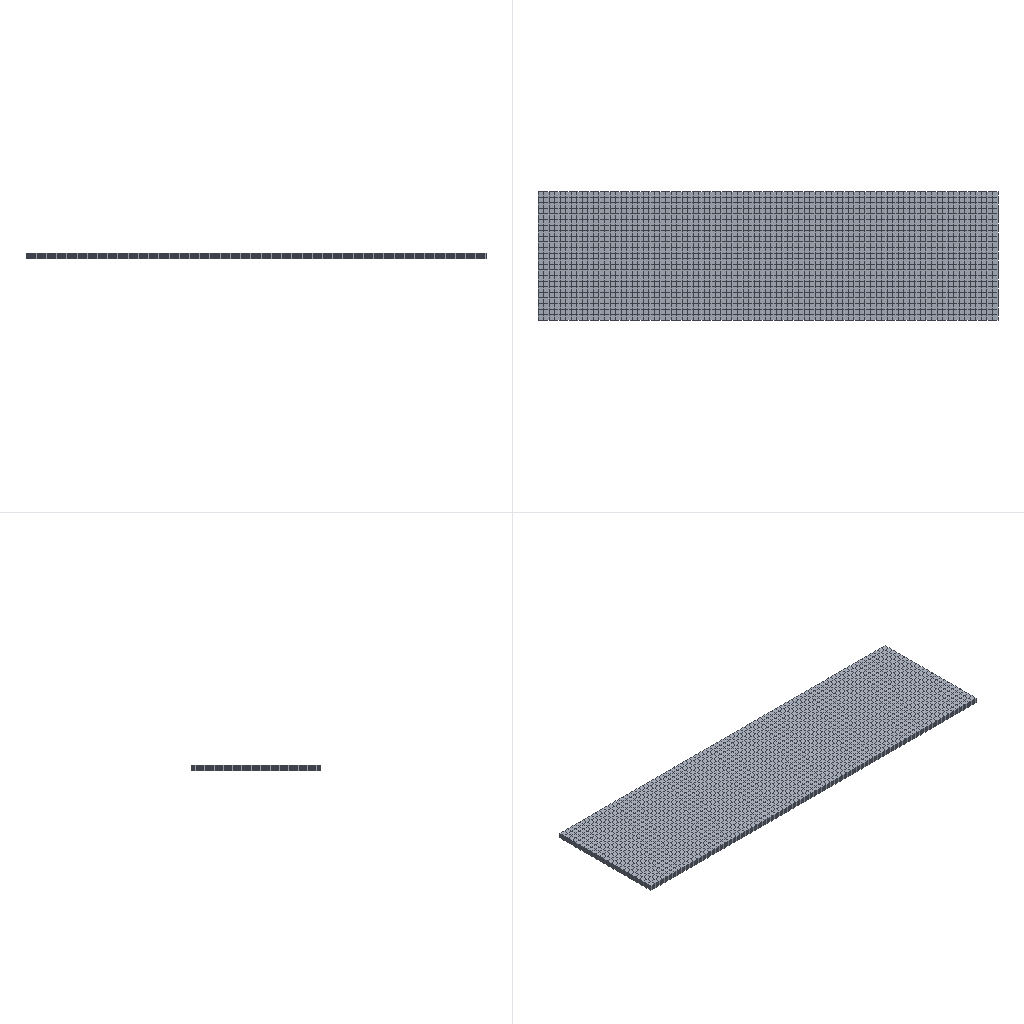Simulation study | abaqus
Set-up summary:
category,name,step,type,value,unit,region
solver,abaqus
solver,version,,,Abaqus/Standard 3DEXPERIENCE R2017x
units,not stated in the deck,,not stated
analysis,deck,,thermal,thermal
load_step,step,step,thermal
load_step,requested,,,1
mesh,nodes,,,12096
mesh,elements,,,9545
element_type,DC3D8,,solid,9545
load,load commands in deck,,count,3
bc,support commands in deck,,count,1
material,SS316,,in results
check,setup vs results,,match,"per instance, exact: element labels, types and connectivity; labels of the nodes the elements use; coordinates of those nodes at SINGLE_PRECISION in 1 of 1 instance(s)"
Abaqus input file, long lists of numbers shortened:
*Heading
** Job name: Job-1 Model name: Job-forming
** Generated by: Abaqus/CAE 2017
*Preprint, echo=NO, model=NO, history=NO, contact=NO
**
** PARTS
**
*Part, name=work
*Node
      1,        1250.,        -350.,          15.
      2,   1234.94,        -350.,          15.
** (12094 more lines like these left out)
*Element, type=DC3D8
   1,   505,   506,   590,   589,     1,     2,    86,    85
   2,   506,   507,   591,   590,     2,     3,    87,    86
** (9543 more lines like these left out)
*Nset, nset=Set-3, generate
     1,  12096,      1
*Elset, elset=Set-3, generate
    1,  9545,     1
** Section: Section-1
*Solid Section, elset=Set-3, material=ss316
,
*End Part
**
**
** ASSEMBLY
**
*Assembly, name=Assembly
**
*Instance, name=work-1, part=work
*End Instance
**
*Nset, nset=Set-32, instance=work-1, generate
     1,  12096,      1
*Elset, elset=Set-32, instance=work-1, generate
    1,  9545,     1
*Nset, nset=Set-48, instance=work-1, generate
     1,  12096,      1
*Elset, elset=Set-48, instance=work-1, generate
    1,  9545,     1
*Nset, nset=Set-49, instance=work-1
     1,     2,     3,     4,     5,     6,     7,     8,     9,    10,    11,    12,    13,    14,    15,    16
    17,    18,    19,    20,    21,    22,    23,    24,    25,    26,    27,    28,    29,    30,    31,    32
** (61 more lines like these left out)
*Elset, elset=Set-49, instance=work-1
    1,    2,    3,    4,    5,    6,    7,    8,    9,   10,   11,   12,   13,   14,   15,   16
   17,   18,   19,   20,   21,   22,   23,   24,   25,   26,   27,   28,   29,   30,   31,   32
** (50 more lines like these left out)
*Nset, nset=Set-50, instance=work-1, generate
     1,  12096,      1
*Elset, elset=Set-50, instance=work-1, generate
    1,  9545,     1
*Elset, elset=_Surf-37_S1, internal, instance=work-1, generate
 9131,  9545,     1
*Elset, elset=_Surf-37_S6, internal, instance=work-1, generate
    1,  9463,    83
*Elset, elset=_Surf-37_S2, internal, instance=work-1, generate
   1,  415,    1
*Elset, elset=_Surf-37_S4, internal, instance=work-1, generate
   83,  9545,    83
*Elset, elset=_Surf-37_S3, internal, instance=work-1
    1,    2,    3,    4,    5,    6,    7,    8,    9,   10,   11,   12,   13,   14,   15,   16
   17,   18,   19,   20,   21,   22,   23,   24,   25,   26,   27,   28,   29,   30,   31,   32
** (118 more lines like these left out)
*Elset, elset=_Surf-37_S5, internal, instance=work-1
  333,  334,  335,  336,  337,  338,  339,  340,  341,  342,  343,  344,  345,  346,  347,  348
  349,  350,  351,  352,  353,  354,  355,  356,  357,  358,  359,  360,  361,  362,  363,  364
** (118 more lines like these left out)
*Surface, type=ELEMENT, name=Surf-37
_Surf-37_S1, S1
_Surf-37_S6, S6
_Surf-37_S2, S2
_Surf-37_S4, S4
_Surf-37_S3, S3
_Surf-37_S5, S5
*Elset, elset=_Surf-38_S1, internal, instance=work-1, generate
 9131,  9545,     1
*Elset, elset=_Surf-38_S6, internal, instance=work-1, generate
    1,  9463,    83
*Elset, elset=_Surf-38_S2, internal, instance=work-1, generate
   1,  415,    1
*Elset, elset=_Surf-38_S4, internal, instance=work-1, generate
   83,  9545,    83
*Elset, elset=_Surf-38_S3, internal, instance=work-1
    1,    2,    3,    4,    5,    6,    7,    8,    9,   10,   11,   12,   13,   14,   15,   16
   17,   18,   19,   20,   21,   22,   23,   24,   25,   26,   27,   28,   29,   30,   31,   32
** (118 more lines like these left out)
*Elset, elset=_Surf-38_S5, internal, instance=work-1
  333,  334,  335,  336,  337,  338,  339,  340,  341,  342,  343,  344,  345,  346,  347,  348
  349,  350,  351,  352,  353,  354,  355,  356,  357,  358,  359,  360,  361,  362,  363,  364
** (118 more lines like these left out)
*Surface, type=ELEMENT, name=Surf-38
_Surf-38_S1, S1
_Surf-38_S6, S6
_Surf-38_S2, S2
_Surf-38_S4, S4
_Surf-38_S3, S3
_Surf-38_S5, S5
*End Assembly
*Amplitude, name=Amp-1
             0.,              1.,             0.1,              1.
**
** MATERIALS
**
*Material, name=ss316
*Conductivity
 13.31,  20.
 16.33, 200.
 19.47, 400.
 22.38, 600.
 25.07, 800.
 26.33, 900.
 27.53,1000.
 28.67,1100.
 29.76,1200.
 31.95,1420.
  320.,1460.
*Density
 7.966e-09,  20.
 7.893e-09, 200.
 7.814e-09, 400.
 7.724e-09, 600.
  7.63e-09, 800.
 7.583e-09, 900.
 7.535e-09,1000.
 7.486e-09,1100.
 7.436e-09,1200.
  7.32e-09,1420.
  7.32e-09,1460.
*Elastic
195100., 0.267,   20.
185700.,  0.29,  200.
172600.,   0.3,  400.
155000., 0.296,  600.
131400., 0.262,  800.
116800.,  0.24,  900.
100100., 0.229, 1000.
 81100., 0.223, 1100.
 59500., 0.223, 1200.
  2000., 0.223, 1420.
  2000., 0.223, 1460.
*Expansion
 1.524e-05,  20.
 1.643e-05, 200.
 1.744e-05, 400.
 1.821e-05, 600.
 1.883e-05, 800.
 1.911e-05, 900.
 1.938e-05,1000.
 1.966e-05,1100.
 1.995e-05,1200.
  2.07e-05,1420.
  2.07e-05,1460.
*Plastic
278.,   0.,  20.
325., 0.01,  20.
193.,   0., 200.
226., 0.01, 200.
154.,   0., 400.
180., 0.01, 400.
141.,   0., 600.
165., 0.01, 600.
130.,   0., 800.
153., 0.01, 800.
 86.,   0., 900.
100., 0.01, 900.
 45.,   0.,1000.
 53., 0.01,1000.
 22.,   0.,1100.
 23., 0.01,1100.
 13.,   0.,1200.
 15., 0.01,1200.
  3.,   0.,1420.
 3.3, 0.01,1420.
  3.,   0.,1460.
 3.3, 0.01,1460.
*Specific Heat
  4.7e+08,  20.
 5.08e+08, 200.
  5.5e+08, 400.
 5.92e+08, 600.
 6.34e+08, 800.
 6.55e+08, 900.
 6.76e+08,1000.
 6.98e+08,1100.
 7.19e+08,1200.
 7.65e+08,1420.
 7.65e+08,1460.
**
** PHYSICAL CONSTANTS
**
*Physical Constants, absolute zero=-273.13, stefan boltzmann=5.67e-08
**
** BOUNDARY CONDITIONS
**
** Name: Disp-BC-1 Type: 对称/反对称/完全固定
*Boundary
Set-49, ENCASTRE
**
** PREDEFINED FIELDS
**
** Name: Predefined Field-1   Type: Temperature
*Initial Conditions, type=TEMPERATURE
Set-50, 950.
** ----------------------------------------------------------------
**
** STEP: step
**
*Step, name=step, nlgeom=NO, inc=1000
*Heat Transfer, end=PERIOD, deltmx=1000.
0.1, 15., 0.00015, 15.,
*Adaptive Mesh Controls, name=Ada-1
1., 0.
**
** LOADS
**
** Name: Load-2   Type: Body heat flux
*Dflux
Set-48, BFNU, 1.
**
** INTERACTIONS
**
** Interaction: SURFFILM-1
*Sfilm
Surf-37, F, 950., 10.
** Interaction: SURFRADIATE-1
*Sradiate
Surf-38, R, 950., 0.4
**
** OUTPUT REQUESTS
**
*Restart, write, frequency=0
**
** FIELD OUTPUT: step
**
*Output, field, number interval=150
*Node Output
NT,
*Element Output, directions=YES
HFL, TEMP
*Output, history, frequency=0
*End Step
Results summary:
result,step,,partial,increments=0 time=0.0/15.0
result,analysis,,,"heat transfer, deltamx"
result,last_loadstep,,,1
result,primary field,,,NT11